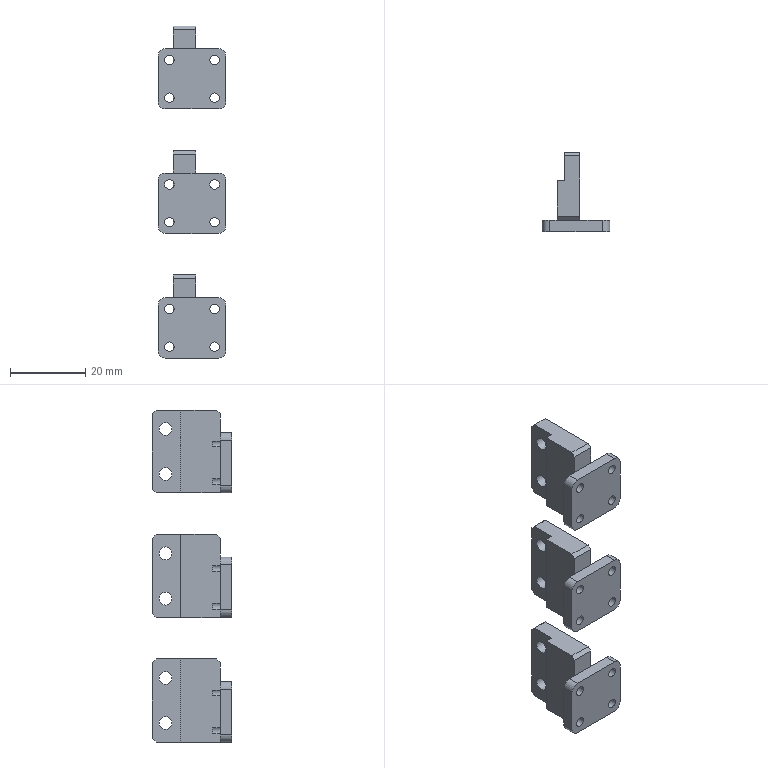Part | 3 solids | 87 faces | box 18 x 21 x 88 mm | volume 8280 mm3 | plane 51 | cylinder 30 | cone 6 | commonest cylinder face diameters 2.5 x12 4 x12 3.4 x6